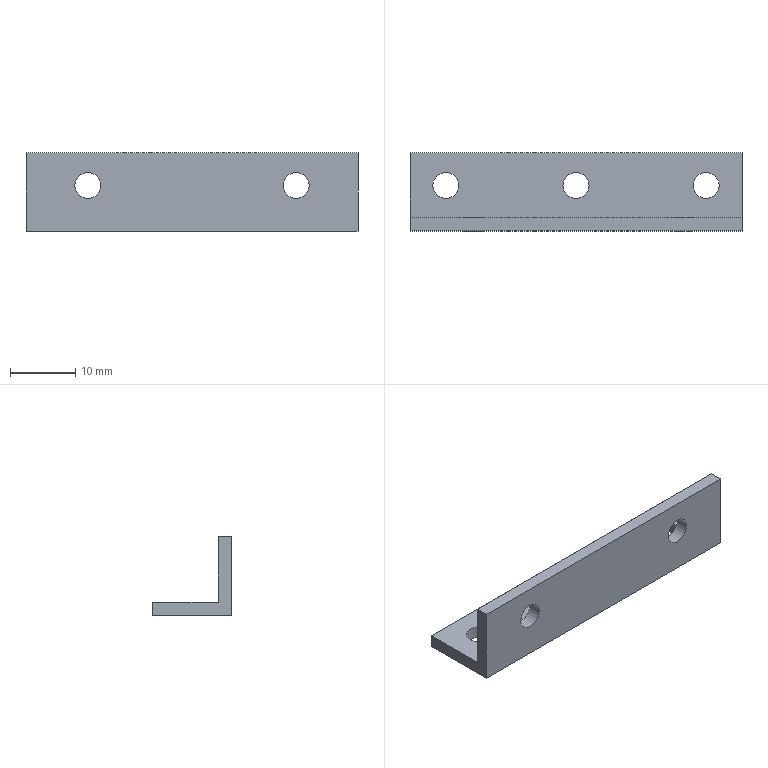Part | STEP file | 1-01.8 | 1 solid | 13 faces | box 51 x 12 x 12 mm | volume 2118 mm3 | plane 8 | cylinder 5 | commonest cylinder face diameters 4 x5
STEP:
#1=CARTESIAN_POINT('',(0.,0.,0.));
#2=DIRECTION('',(0.,0.,1.));
#3=DIRECTION('',(1.,0.,0.));
#4=AXIS2_PLACEMENT_3D('',#1,#2,#3);
#5=CARTESIAN_POINT('',(25.5,-6.,-6.));
#6=VERTEX_POINT('',#5);
#7=CARTESIAN_POINT('',(25.5,6.,-6.));
#8=VERTEX_POINT('',#7);
#9=CARTESIAN_POINT('',(25.5,-6.,-6.));
#10=DIRECTION('',(0.,1.,0.));
#11=VECTOR('',#10,1.);
#12=LINE('',#9,#11);
#13=CARTESIAN_POINT('',(25.5,0.,0.));
#14=DIRECTION('',(1.,0.,0.));
#15=DIRECTION('',(0.,1.,0.));
#16=AXIS2_PLACEMENT_3D('',#13,#14,#15);
#17=PLANE('',#16);
#18=CARTESIAN_POINT('',(-6.,-6.));
#19=DIRECTION('',(1.,0.));
#20=VECTOR('',#19,1.);
#21=LINE('',#18,#20);
#22=(GEOMETRIC_REPRESENTATION_CONTEXT(2)PARAMETRIC_REPRESENTATION_CONTEXT()REPRESENTATION_CONTEXT('',''));
#23=DEFINITIONAL_REPRESENTATION('',(#21),#22);
#24=PCURVE('',#17,#23);
#25=CARTESIAN_POINT('',(0.,0.,-6.));
#26=DIRECTION('',(0.,0.,1.));
#27=DIRECTION('',(0.,1.,0.));
#28=AXIS2_PLACEMENT_3D('',#25,#26,#27);
#29=PLANE('',#28);
#30=CARTESIAN_POINT('',(-6.,-25.5));
#31=DIRECTION('',(1.,0.));
#32=VECTOR('',#31,1.);
#33=LINE('',#30,#32);
#34=(GEOMETRIC_REPRESENTATION_CONTEXT(2)PARAMETRIC_REPRESENTATION_CONTEXT()REPRESENTATION_CONTEXT('',''));
#35=DEFINITIONAL_REPRESENTATION('',(#33),#34);
#36=PCURVE('',#29,#35);
#37=SURFACE_CURVE('',#12,(#24,#36),.PCURVE_S1.);
#38=EDGE_CURVE('',#6,#8,#37,.T.);
#39=ORIENTED_EDGE('',*,*,#38,.T.);
#40=CARTESIAN_POINT('',(25.5,6.,-4.));
#41=VERTEX_POINT('',#40);
#42=CARTESIAN_POINT('',(25.5,6.,-6.));
#43=DIRECTION('',(0.,0.,1.));
#44=VECTOR('',#43,1.);
#45=LINE('',#42,#44);
#46=CARTESIAN_POINT('',(6.,-6.));
#47=DIRECTION('',(0.,1.));
#48=VECTOR('',#47,1.);
#49=LINE('',#46,#48);
#50=(GEOMETRIC_REPRESENTATION_CONTEXT(2)PARAMETRIC_REPRESENTATION_CONTEXT()REPRESENTATION_CONTEXT('',''));
#51=DEFINITIONAL_REPRESENTATION('',(#49),#50);
#52=PCURVE('',#17,#51);
#53=CARTESIAN_POINT('',(0.,6.,-5.));
#54=DIRECTION('',(0.,-1.,0.));
#55=DIRECTION('',(0.,0.,1.));
#56=AXIS2_PLACEMENT_3D('',#53,#54,#55);
#57=PLANE('',#56);
#58=CARTESIAN_POINT('',(-1.,-25.5));
#59=DIRECTION('',(1.,0.));
#60=VECTOR('',#59,1.);
#61=LINE('',#58,#60);
#62=(GEOMETRIC_REPRESENTATION_CONTEXT(2)PARAMETRIC_REPRESENTATION_CONTEXT()REPRESENTATION_CONTEXT('',''));
#63=DEFINITIONAL_REPRESENTATION('',(#61),#62);
#64=PCURVE('',#57,#63);
#65=SURFACE_CURVE('',#45,(#52,#64),.PCURVE_S1.);
#66=EDGE_CURVE('',#8,#41,#65,.T.);
#67=ORIENTED_EDGE('',*,*,#66,.T.);
#68=CARTESIAN_POINT('',(25.5,-4.,-4.));
#69=VERTEX_POINT('',#68);
#70=CARTESIAN_POINT('',(25.5,6.,-4.));
#71=DIRECTION('',(0.,-1.,0.));
#72=VECTOR('',#71,1.);
#73=LINE('',#70,#72);
#74=CARTESIAN_POINT('',(6.,-4.));
#75=DIRECTION('',(-1.,0.));
#76=VECTOR('',#75,1.);
#77=LINE('',#74,#76);
#78=(GEOMETRIC_REPRESENTATION_CONTEXT(2)PARAMETRIC_REPRESENTATION_CONTEXT()REPRESENTATION_CONTEXT('',''));
#79=DEFINITIONAL_REPRESENTATION('',(#77),#78);
#80=PCURVE('',#17,#79);
#81=CARTESIAN_POINT('',(0.,1.,-4.));
#82=DIRECTION('',(0.,0.,-1.));
#83=DIRECTION('',(0.,-1.,0.));
#84=AXIS2_PLACEMENT_3D('',#81,#82,#83);
#85=PLANE('',#84);
#86=CARTESIAN_POINT('',(-5.,-25.5));
#87=DIRECTION('',(1.,0.));
#88=VECTOR('',#87,1.);
#89=LINE('',#86,#88);
#90=(GEOMETRIC_REPRESENTATION_CONTEXT(2)PARAMETRIC_REPRESENTATION_CONTEXT()REPRESENTATION_CONTEXT('',''));
#91=DEFINITIONAL_REPRESENTATION('',(#89),#90);
#92=PCURVE('',#85,#91);
#93=SURFACE_CURVE('',#73,(#80,#92),.PCURVE_S1.);
#94=EDGE_CURVE('',#41,#69,#93,.T.);
#95=ORIENTED_EDGE('',*,*,#94,.T.);
#96=CARTESIAN_POINT('',(25.5,-4.,6.));
#97=VERTEX_POINT('',#96);
#98=CARTESIAN_POINT('',(25.5,-4.,-4.));
#99=DIRECTION('',(0.,0.,1.));
#100=VECTOR('',#99,1.);
#101=LINE('',#98,#100);
#102=CARTESIAN_POINT('',(-4.,-4.));
#103=DIRECTION('',(0.,1.));
#104=VECTOR('',#103,1.);
#105=LINE('',#102,#104);
#106=(GEOMETRIC_REPRESENTATION_CONTEXT(2)PARAMETRIC_REPRESENTATION_CONTEXT()REPRESENTATION_CONTEXT('',''));
#107=DEFINITIONAL_REPRESENTATION('',(#105),#106);
#108=PCURVE('',#17,#107);
#109=CARTESIAN_POINT('',(0.,-4.,1.));
#110=DIRECTION('',(0.,-1.,0.));
#111=DIRECTION('',(0.,0.,1.));
#112=AXIS2_PLACEMENT_3D('',#109,#110,#111);
#113=PLANE('',#112);
#114=CARTESIAN_POINT('',(-5.,-25.5));
#115=DIRECTION('',(1.,0.));
#116=VECTOR('',#115,1.);
#117=LINE('',#114,#116);
#118=(GEOMETRIC_REPRESENTATION_CONTEXT(2)PARAMETRIC_REPRESENTATION_CONTEXT()REPRESENTATION_CONTEXT('',''));
#119=DEFINITIONAL_REPRESENTATION('',(#117),#118);
#120=PCURVE('',#113,#119);
#121=SURFACE_CURVE('',#101,(#108,#120),.PCURVE_S1.);
#122=EDGE_CURVE('',#69,#97,#121,.T.);
#123=ORIENTED_EDGE('',*,*,#122,.T.);
#124=CARTESIAN_POINT('',(25.5,-6.,6.));
#125=VERTEX_POINT('',#124);
#126=CARTESIAN_POINT('',(25.5,-4.,6.));
#127=DIRECTION('',(0.,-1.,0.));
#128=VECTOR('',#127,1.);
#129=LINE('',#126,#128);
#130=CARTESIAN_POINT('',(-4.,6.));
#131=DIRECTION('',(-1.,0.));
#132=VECTOR('',#131,1.);
#133=LINE('',#130,#132);
#134=(GEOMETRIC_REPRESENTATION_CONTEXT(2)PARAMETRIC_REPRESENTATION_CONTEXT()REPRESENTATION_CONTEXT('',''));
#135=DEFINITIONAL_REPRESENTATION('',(#133),#134);
#136=PCURVE('',#17,#135);
#137=CARTESIAN_POINT('',(0.,-5.,6.));
#138=DIRECTION('',(0.,0.,-1.));
#139=DIRECTION('',(0.,-1.,0.));
#140=AXIS2_PLACEMENT_3D('',#137,#138,#139);
#141=PLANE('',#140);
#142=CARTESIAN_POINT('',(-1.,-25.5));
#143=DIRECTION('',(1.,0.));
#144=VECTOR('',#143,1.);
#145=LINE('',#142,#144);
#146=(GEOMETRIC_REPRESENTATION_CONTEXT(2)PARAMETRIC_REPRESENTATION_CONTEXT()REPRESENTATION_CONTEXT('',''));
#147=DEFINITIONAL_REPRESENTATION('',(#145),#146);
#148=PCURVE('',#141,#147);
#149=SURFACE_CURVE('',#129,(#136,#148),.PCURVE_S1.);
#150=EDGE_CURVE('',#97,#125,#149,.T.);
#151=ORIENTED_EDGE('',*,*,#150,.T.);
#152=CARTESIAN_POINT('',(25.5,-6.,6.));
#153=DIRECTION('',(0.,0.,-1.));
#154=VECTOR('',#153,1.);
#155=LINE('',#152,#154);
#156=CARTESIAN_POINT('',(-6.,6.));
#157=DIRECTION('',(0.,-1.));
#158=VECTOR('',#157,1.);
#159=LINE('',#156,#158);
#160=(GEOMETRIC_REPRESENTATION_CONTEXT(2)PARAMETRIC_REPRESENTATION_CONTEXT()REPRESENTATION_CONTEXT('',''));
#161=DEFINITIONAL_REPRESENTATION('',(#159),#160);
#162=PCURVE('',#17,#161);
#163=CARTESIAN_POINT('',(0.,-6.,0.));
#164=DIRECTION('',(0.,1.,0.));
#165=DIRECTION('',(0.,0.,-1.));
#166=AXIS2_PLACEMENT_3D('',#163,#164,#165);
#167=PLANE('',#166);
#168=CARTESIAN_POINT('',(-6.,-25.5));
#169=DIRECTION('',(1.,0.));
#170=VECTOR('',#169,1.);
#171=LINE('',#168,#170);
#172=(GEOMETRIC_REPRESENTATION_CONTEXT(2)PARAMETRIC_REPRESENTATION_CONTEXT()REPRESENTATION_CONTEXT('',''));
#173=DEFINITIONAL_REPRESENTATION('',(#171),#172);
#174=PCURVE('',#167,#173);
#175=SURFACE_CURVE('',#155,(#162,#174),.PCURVE_S1.);
#176=EDGE_CURVE('',#125,#6,#175,.T.);
#177=ORIENTED_EDGE('',*,*,#176,.T.);
#178=EDGE_LOOP('',(#39,#67,#95,#123,#151,#177));
#179=FACE_BOUND('',#178,.T.);
#180=ADVANCED_FACE('',(#179),#17,.T.);
#181=CARTESIAN_POINT('',(-25.5,-6.,-6.));
#182=VERTEX_POINT('',#181);
#183=CARTESIAN_POINT('',(-25.5,6.,-6.));
#184=VERTEX_POINT('',#183);
#185=CARTESIAN_POINT('',(-25.5,-6.,-6.));
#186=DIRECTION('',(0.,1.,0.));
#187=VECTOR('',#186,1.);
#188=LINE('',#185,#187);
#189=CARTESIAN_POINT('',(-25.5,0.,0.));
#190=DIRECTION('',(1.,0.,0.));
#191=DIRECTION('',(0.,1.,0.));
#192=AXIS2_PLACEMENT_3D('',#189,#190,#191);
#193=PLANE('',#192);
#194=CARTESIAN_POINT('',(-6.,-6.));
#195=DIRECTION('',(1.,0.));
#196=VECTOR('',#195,1.);
#197=LINE('',#194,#196);
#198=(GEOMETRIC_REPRESENTATION_CONTEXT(2)PARAMETRIC_REPRESENTATION_CONTEXT()REPRESENTATION_CONTEXT('',''));
#199=DEFINITIONAL_REPRESENTATION('',(#197),#198);
#200=PCURVE('',#193,#199);
#201=CARTESIAN_POINT('',(-6.,25.5));
#202=DIRECTION('',(1.,0.));
#203=VECTOR('',#202,1.);
#204=LINE('',#201,#203);
#205=(GEOMETRIC_REPRESENTATION_CONTEXT(2)PARAMETRIC_REPRESENTATION_CONTEXT()REPRESENTATION_CONTEXT('',''));
#206=DEFINITIONAL_REPRESENTATION('',(#204),#205);
#207=PCURVE('',#29,#206);
#208=SURFACE_CURVE('',#188,(#200,#207),.PCURVE_S1.);
#209=EDGE_CURVE('',#182,#184,#208,.T.);
#210=ORIENTED_EDGE('',*,*,#209,.T.);
#211=CARTESIAN_POINT('',(-25.5,6.,-4.));
#212=VERTEX_POINT('',#211);
#213=CARTESIAN_POINT('',(-25.5,6.,-6.));
#214=DIRECTION('',(0.,0.,1.));
#215=VECTOR('',#214,1.);
#216=LINE('',#213,#215);
#217=CARTESIAN_POINT('',(6.,-6.));
#218=DIRECTION('',(0.,1.));
#219=VECTOR('',#218,1.);
#220=LINE('',#217,#219);
#221=(GEOMETRIC_REPRESENTATION_CONTEXT(2)PARAMETRIC_REPRESENTATION_CONTEXT()REPRESENTATION_CONTEXT('',''));
#222=DEFINITIONAL_REPRESENTATION('',(#220),#221);
#223=PCURVE('',#193,#222);
#224=CARTESIAN_POINT('',(-1.,25.5));
#225=DIRECTION('',(1.,0.));
#226=VECTOR('',#225,1.);
#227=LINE('',#224,#226);
#228=(GEOMETRIC_REPRESENTATION_CONTEXT(2)PARAMETRIC_REPRESENTATION_CONTEXT()REPRESENTATION_CONTEXT('',''));
#229=DEFINITIONAL_REPRESENTATION('',(#227),#228);
#230=PCURVE('',#57,#229);
#231=SURFACE_CURVE('',#216,(#223,#230),.PCURVE_S1.);
#232=EDGE_CURVE('',#184,#212,#231,.T.);
#233=ORIENTED_EDGE('',*,*,#232,.T.);
#234=CARTESIAN_POINT('',(-25.5,-4.,-4.));
#235=VERTEX_POINT('',#234);
#236=CARTESIAN_POINT('',(-25.5,6.,-4.));
#237=DIRECTION('',(0.,-1.,0.));
#238=VECTOR('',#237,1.);
#239=LINE('',#236,#238);
#240=CARTESIAN_POINT('',(6.,-4.));
#241=DIRECTION('',(-1.,0.));
#242=VECTOR('',#241,1.);
#243=LINE('',#240,#242);
#244=(GEOMETRIC_REPRESENTATION_CONTEXT(2)PARAMETRIC_REPRESENTATION_CONTEXT()REPRESENTATION_CONTEXT('',''));
#245=DEFINITIONAL_REPRESENTATION('',(#243),#244);
#246=PCURVE('',#193,#245);
#247=CARTESIAN_POINT('',(-5.,25.5));
#248=DIRECTION('',(1.,0.));
#249=VECTOR('',#248,1.);
#250=LINE('',#247,#249);
#251=(GEOMETRIC_REPRESENTATION_CONTEXT(2)PARAMETRIC_REPRESENTATION_CONTEXT()REPRESENTATION_CONTEXT('',''));
#252=DEFINITIONAL_REPRESENTATION('',(#250),#251);
#253=PCURVE('',#85,#252);
#254=SURFACE_CURVE('',#239,(#246,#253),.PCURVE_S1.);
#255=EDGE_CURVE('',#212,#235,#254,.T.);
#256=ORIENTED_EDGE('',*,*,#255,.T.);
#257=CARTESIAN_POINT('',(-25.5,-4.,6.));
#258=VERTEX_POINT('',#257);
#259=CARTESIAN_POINT('',(-25.5,-4.,-4.));
#260=DIRECTION('',(0.,0.,1.));
#261=VECTOR('',#260,1.);
#262=LINE('',#259,#261);
#263=CARTESIAN_POINT('',(-4.,-4.));
#264=DIRECTION('',(0.,1.));
#265=VECTOR('',#264,1.);
#266=LINE('',#263,#265);
#267=(GEOMETRIC_REPRESENTATION_CONTEXT(2)PARAMETRIC_REPRESENTATION_CONTEXT()REPRESENTATION_CONTEXT('',''));
#268=DEFINITIONAL_REPRESENTATION('',(#266),#267);
#269=PCURVE('',#193,#268);
#270=CARTESIAN_POINT('',(-5.,25.5));
#271=DIRECTION('',(1.,0.));
#272=VECTOR('',#271,1.);
#273=LINE('',#270,#272);
#274=(GEOMETRIC_REPRESENTATION_CONTEXT(2)PARAMETRIC_REPRESENTATION_CONTEXT()REPRESENTATION_CONTEXT('',''));
#275=DEFINITIONAL_REPRESENTATION('',(#273),#274);
#276=PCURVE('',#113,#275);
#277=SURFACE_CURVE('',#262,(#269,#276),.PCURVE_S1.);
#278=EDGE_CURVE('',#235,#258,#277,.T.);
#279=ORIENTED_EDGE('',*,*,#278,.T.);
#280=CARTESIAN_POINT('',(-25.5,-6.,6.));
#281=VERTEX_POINT('',#280);
#282=CARTESIAN_POINT('',(-25.5,-4.,6.));
#283=DIRECTION('',(0.,-1.,0.));
#284=VECTOR('',#283,1.);
#285=LINE('',#282,#284);
#286=CARTESIAN_POINT('',(-4.,6.));
#287=DIRECTION('',(-1.,0.));
#288=VECTOR('',#287,1.);
#289=LINE('',#286,#288);
#290=(GEOMETRIC_REPRESENTATION_CONTEXT(2)PARAMETRIC_REPRESENTATION_CONTEXT()REPRESENTATION_CONTEXT('',''));
#291=DEFINITIONAL_REPRESENTATION('',(#289),#290);
#292=PCURVE('',#193,#291);
#293=CARTESIAN_POINT('',(-1.,25.5));
#294=DIRECTION('',(1.,0.));
#295=VECTOR('',#294,1.);
#296=LINE('',#293,#295);
#297=(GEOMETRIC_REPRESENTATION_CONTEXT(2)PARAMETRIC_REPRESENTATION_CONTEXT()REPRESENTATION_CONTEXT('',''));
#298=DEFINITIONAL_REPRESENTATION('',(#296),#297);
#299=PCURVE('',#141,#298);
#300=SURFACE_CURVE('',#285,(#292,#299),.PCURVE_S1.);
#301=EDGE_CURVE('',#258,#281,#300,.T.);
#302=ORIENTED_EDGE('',*,*,#301,.T.);
#303=CARTESIAN_POINT('',(-25.5,-6.,6.));
#304=DIRECTION('',(0.,0.,-1.));
#305=VECTOR('',#304,1.);
#306=LINE('',#303,#305);
#307=CARTESIAN_POINT('',(-6.,6.));
#308=DIRECTION('',(0.,-1.));
#309=VECTOR('',#308,1.);
#310=LINE('',#307,#309);
#311=(GEOMETRIC_REPRESENTATION_CONTEXT(2)PARAMETRIC_REPRESENTATION_CONTEXT()REPRESENTATION_CONTEXT('',''));
#312=DEFINITIONAL_REPRESENTATION('',(#310),#311);
#313=PCURVE('',#193,#312);
#314=CARTESIAN_POINT('',(-6.,25.5));
#315=DIRECTION('',(1.,0.));
#316=VECTOR('',#315,1.);
#317=LINE('',#314,#316);
#318=(GEOMETRIC_REPRESENTATION_CONTEXT(2)PARAMETRIC_REPRESENTATION_CONTEXT()REPRESENTATION_CONTEXT('',''));
#319=DEFINITIONAL_REPRESENTATION('',(#317),#318);
#320=PCURVE('',#167,#319);
#321=SURFACE_CURVE('',#306,(#313,#320),.PCURVE_S1.);
#322=EDGE_CURVE('',#281,#182,#321,.T.);
#323=ORIENTED_EDGE('',*,*,#322,.T.);
#324=EDGE_LOOP('',(#210,#233,#256,#279,#302,#323));
#325=FACE_BOUND('',#324,.F.);
#326=ADVANCED_FACE('',(#325),#193,.F.);
#327=ORIENTED_EDGE('',*,*,#66,.T.);
#328=CARTESIAN_POINT('',(25.5,6.,-4.));
#329=DIRECTION('',(-1.,0.,0.));
#330=VECTOR('',#329,1.);
#331=LINE('',#328,#330);
#332=CARTESIAN_POINT('',(1.,-25.5));
#333=DIRECTION('',(0.,1.));
#334=VECTOR('',#333,1.);
#335=LINE('',#332,#334);
#336=(GEOMETRIC_REPRESENTATION_CONTEXT(2)PARAMETRIC_REPRESENTATION_CONTEXT()REPRESENTATION_CONTEXT('',''));
#337=DEFINITIONAL_REPRESENTATION('',(#335),#336);
#338=PCURVE('',#57,#337);
#339=CARTESIAN_POINT('',(-5.,-25.5));
#340=DIRECTION('',(0.,1.));
#341=VECTOR('',#340,1.);
#342=LINE('',#339,#341);
#343=(GEOMETRIC_REPRESENTATION_CONTEXT(2)PARAMETRIC_REPRESENTATION_CONTEXT()REPRESENTATION_CONTEXT('',''));
#344=DEFINITIONAL_REPRESENTATION('',(#342),#343);
#345=PCURVE('',#85,#344);
#346=SURFACE_CURVE('',#331,(#338,#345),.PCURVE_S1.);
#347=EDGE_CURVE('',#41,#212,#346,.T.);
#348=ORIENTED_EDGE('',*,*,#347,.T.);
#349=ORIENTED_EDGE('',*,*,#232,.F.);
#350=CARTESIAN_POINT('',(25.5,6.,-6.));
#351=DIRECTION('',(-1.,0.,0.));
#352=VECTOR('',#351,1.);
#353=LINE('',#350,#352);
#354=CARTESIAN_POINT('',(-1.,-25.5));
#355=DIRECTION('',(0.,1.));
#356=VECTOR('',#355,1.);
#357=LINE('',#354,#356);
#358=(GEOMETRIC_REPRESENTATION_CONTEXT(2)PARAMETRIC_REPRESENTATION_CONTEXT()REPRESENTATION_CONTEXT('',''));
#359=DEFINITIONAL_REPRESENTATION('',(#357),#358);
#360=PCURVE('',#57,#359);
#361=CARTESIAN_POINT('',(6.,-25.5));
#362=DIRECTION('',(0.,1.));
#363=VECTOR('',#362,1.);
#364=LINE('',#361,#363);
#365=(GEOMETRIC_REPRESENTATION_CONTEXT(2)PARAMETRIC_REPRESENTATION_CONTEXT()REPRESENTATION_CONTEXT('',''));
#366=DEFINITIONAL_REPRESENTATION('',(#364),#365);
#367=PCURVE('',#29,#366);
#368=SURFACE_CURVE('',#353,(#360,#367),.PCURVE_S1.);
#369=EDGE_CURVE('',#8,#184,#368,.T.);
#370=ORIENTED_EDGE('',*,*,#369,.F.);
#371=EDGE_LOOP('',(#327,#348,#349,#370));
#372=FACE_BOUND('',#371,.F.);
#373=ADVANCED_FACE('',(#372),#57,.F.);
#374=ORIENTED_EDGE('',*,*,#150,.T.);
#375=CARTESIAN_POINT('',(25.5,-6.,6.));
#376=DIRECTION('',(-1.,0.,0.));
#377=VECTOR('',#376,1.);
#378=LINE('',#375,#377);
#379=CARTESIAN_POINT('',(1.,-25.5));
#380=DIRECTION('',(0.,1.));
#381=VECTOR('',#380,1.);
#382=LINE('',#379,#381);
#383=(GEOMETRIC_REPRESENTATION_CONTEXT(2)PARAMETRIC_REPRESENTATION_CONTEXT()REPRESENTATION_CONTEXT('',''));
#384=DEFINITIONAL_REPRESENTATION('',(#382),#383);
#385=PCURVE('',#141,#384);
#386=CARTESIAN_POINT('',(-6.,-25.5));
#387=DIRECTION('',(0.,1.));
#388=VECTOR('',#387,1.);
#389=LINE('',#386,#388);
#390=(GEOMETRIC_REPRESENTATION_CONTEXT(2)PARAMETRIC_REPRESENTATION_CONTEXT()REPRESENTATION_CONTEXT('',''));
#391=DEFINITIONAL_REPRESENTATION('',(#389),#390);
#392=PCURVE('',#167,#391);
#393=SURFACE_CURVE('',#378,(#385,#392),.PCURVE_S1.);
#394=EDGE_CURVE('',#125,#281,#393,.T.);
#395=ORIENTED_EDGE('',*,*,#394,.T.);
#396=ORIENTED_EDGE('',*,*,#301,.F.);
#397=CARTESIAN_POINT('',(25.5,-4.,6.));
#398=DIRECTION('',(-1.,0.,0.));
#399=VECTOR('',#398,1.);
#400=LINE('',#397,#399);
#401=CARTESIAN_POINT('',(-1.,-25.5));
#402=DIRECTION('',(0.,1.));
#403=VECTOR('',#402,1.);
#404=LINE('',#401,#403);
#405=(GEOMETRIC_REPRESENTATION_CONTEXT(2)PARAMETRIC_REPRESENTATION_CONTEXT()REPRESENTATION_CONTEXT('',''));
#406=DEFINITIONAL_REPRESENTATION('',(#404),#405);
#407=PCURVE('',#141,#406);
#408=CARTESIAN_POINT('',(5.,-25.5));
#409=DIRECTION('',(0.,1.));
#410=VECTOR('',#409,1.);
#411=LINE('',#408,#410);
#412=(GEOMETRIC_REPRESENTATION_CONTEXT(2)PARAMETRIC_REPRESENTATION_CONTEXT()REPRESENTATION_CONTEXT('',''));
#413=DEFINITIONAL_REPRESENTATION('',(#411),#412);
#414=PCURVE('',#113,#413);
#415=SURFACE_CURVE('',#400,(#407,#414),.PCURVE_S1.);
#416=EDGE_CURVE('',#97,#258,#415,.T.);
#417=ORIENTED_EDGE('',*,*,#416,.F.);
#418=EDGE_LOOP('',(#374,#395,#396,#417));
#419=FACE_BOUND('',#418,.F.);
#420=ADVANCED_FACE('',(#419),#141,.F.);
#421=ORIENTED_EDGE('',*,*,#122,.T.);
#422=ORIENTED_EDGE('',*,*,#416,.T.);
#423=ORIENTED_EDGE('',*,*,#278,.F.);
#424=CARTESIAN_POINT('',(25.5,-4.,-4.));
#425=DIRECTION('',(-1.,0.,0.));
#426=VECTOR('',#425,1.);
#427=LINE('',#424,#426);
#428=CARTESIAN_POINT('',(-5.,-25.5));
#429=DIRECTION('',(0.,1.));
#430=VECTOR('',#429,1.);
#431=LINE('',#428,#430);
#432=(GEOMETRIC_REPRESENTATION_CONTEXT(2)PARAMETRIC_REPRESENTATION_CONTEXT()REPRESENTATION_CONTEXT('',''));
#433=DEFINITIONAL_REPRESENTATION('',(#431),#432);
#434=PCURVE('',#113,#433);
#435=CARTESIAN_POINT('',(5.,-25.5));
#436=DIRECTION('',(0.,1.));
#437=VECTOR('',#436,1.);
#438=LINE('',#435,#437);
#439=(GEOMETRIC_REPRESENTATION_CONTEXT(2)PARAMETRIC_REPRESENTATION_CONTEXT()REPRESENTATION_CONTEXT('',''));
#440=DEFINITIONAL_REPRESENTATION('',(#438),#439);
#441=PCURVE('',#85,#440);
#442=SURFACE_CURVE('',#427,(#434,#441),.PCURVE_S1.);
#443=EDGE_CURVE('',#69,#235,#442,.T.);
#444=ORIENTED_EDGE('',*,*,#443,.F.);
#445=EDGE_LOOP('',(#421,#422,#423,#444));
#446=FACE_BOUND('',#445,.F.);
#447=CARTESIAN_POINT('',(-14.,-4.,1.));
#448=VERTEX_POINT('',#447);
#449=CARTESIAN_POINT('',(-16.,-4.,1.));
#450=DIRECTION('',(0.,1.,0.));
#451=DIRECTION('',(1.,0.,0.));
#452=AXIS2_PLACEMENT_3D('',#449,#450,#451);
#453=CIRCLE('',#452,2.);
#454=CARTESIAN_POINT('',(0.,14.));
#455=CARTESIAN_POINT('',(-3.464,14.));
#456=CARTESIAN_POINT('',(-1.732,17.));
#457=CARTESIAN_POINT('',(0.,20.));
#458=CARTESIAN_POINT('',(1.732,17.));
#459=CARTESIAN_POINT('',(3.464,14.));
#460=CARTESIAN_POINT('',(0.,14.));
#461=(BOUNDED_CURVE()B_SPLINE_CURVE(2,(#454,#455,#456,#457,#458,#459,#460),.UNSPECIFIED.,.T.,.F.)B_SPLINE_CURVE_WITH_KNOTS((1,2,2,2,2,1),(-2.094,0.,2.094,4.189,6.283,8.378),.UNSPECIFIED.)CURVE()GEOMETRIC_REPRESENTATION_ITEM()RATIONAL_B_SPLINE_CURVE((1.,0.5,1.,0.5,1.,0.5,1.))REPRESENTATION_ITEM(''));
#462=(GEOMETRIC_REPRESENTATION_CONTEXT(2)PARAMETRIC_REPRESENTATION_CONTEXT()REPRESENTATION_CONTEXT('',''));
#463=DEFINITIONAL_REPRESENTATION('',(#461),#462);
#464=PCURVE('',#113,#463);
#465=CARTESIAN_POINT('',(-16.,-25.5,1.));
#466=DIRECTION('',(0.,1.,0.));
#467=DIRECTION('',(1.,0.,0.));
#468=AXIS2_PLACEMENT_3D('',#465,#466,#467);
#469=CYLINDRICAL_SURFACE('',#468,2.);
#470=CARTESIAN_POINT('',(0.,21.5));
#471=DIRECTION('',(1.,0.));
#472=VECTOR('',#471,1.);
#473=LINE('',#470,#472);
#474=(GEOMETRIC_REPRESENTATION_CONTEXT(2)PARAMETRIC_REPRESENTATION_CONTEXT()REPRESENTATION_CONTEXT('',''));
#475=DEFINITIONAL_REPRESENTATION('',(#473),#474);
#476=PCURVE('',#469,#475);
#477=SURFACE_CURVE('',#453,(#464,#476),.PCURVE_S1.);
#478=EDGE_CURVE('',#448,#448,#477,.T.);
#479=ORIENTED_EDGE('',*,*,#478,.T.);
#480=EDGE_LOOP('',(#479));
#481=FACE_BOUND('',#480,.F.);
#482=CARTESIAN_POINT('',(18.,-4.,1.));
#483=VERTEX_POINT('',#482);
#484=CARTESIAN_POINT('',(16.,-4.,1.));
#485=DIRECTION('',(0.,1.,0.));
#486=DIRECTION('',(1.,0.,0.));
#487=AXIS2_PLACEMENT_3D('',#484,#485,#486);
#488=CIRCLE('',#487,2.);
#489=CARTESIAN_POINT('',(0.,-18.));
#490=CARTESIAN_POINT('',(-3.464,-18.));
#491=CARTESIAN_POINT('',(-1.732,-15.));
#492=CARTESIAN_POINT('',(0.,-12.));
#493=CARTESIAN_POINT('',(1.732,-15.));
#494=CARTESIAN_POINT('',(3.464,-18.));
#495=CARTESIAN_POINT('',(0.,-18.));
#496=(BOUNDED_CURVE()B_SPLINE_CURVE(2,(#489,#490,#491,#492,#493,#494,#495),.UNSPECIFIED.,.T.,.F.)B_SPLINE_CURVE_WITH_KNOTS((1,2,2,2,2,1),(-2.094,0.,2.094,4.189,6.283,8.378),.UNSPECIFIED.)CURVE()GEOMETRIC_REPRESENTATION_ITEM()RATIONAL_B_SPLINE_CURVE((1.,0.5,1.,0.5,1.,0.5,1.))REPRESENTATION_ITEM(''));
#497=(GEOMETRIC_REPRESENTATION_CONTEXT(2)PARAMETRIC_REPRESENTATION_CONTEXT()REPRESENTATION_CONTEXT('',''));
#498=DEFINITIONAL_REPRESENTATION('',(#496),#497);
#499=PCURVE('',#113,#498);
#500=CARTESIAN_POINT('',(16.,-25.5,1.));
#501=DIRECTION('',(0.,1.,0.));
#502=DIRECTION('',(1.,0.,0.));
#503=AXIS2_PLACEMENT_3D('',#500,#501,#502);
#504=CYLINDRICAL_SURFACE('',#503,2.);
#505=CARTESIAN_POINT('',(0.,21.5));
#506=DIRECTION('',(1.,0.));
#507=VECTOR('',#506,1.);
#508=LINE('',#505,#507);
#509=(GEOMETRIC_REPRESENTATION_CONTEXT(2)PARAMETRIC_REPRESENTATION_CONTEXT()REPRESENTATION_CONTEXT('',''));
#510=DEFINITIONAL_REPRESENTATION('',(#508),#509);
#511=PCURVE('',#504,#510);
#512=SURFACE_CURVE('',#488,(#499,#511),.PCURVE_S1.);
#513=EDGE_CURVE('',#483,#483,#512,.T.);
#514=ORIENTED_EDGE('',*,*,#513,.T.);
#515=EDGE_LOOP('',(#514));
#516=FACE_BOUND('',#515,.F.);
#517=ADVANCED_FACE('',(#446,#481,#516),#113,.F.);
#518=ORIENTED_EDGE('',*,*,#176,.T.);
#519=CARTESIAN_POINT('',(25.5,-6.,-6.));
#520=DIRECTION('',(-1.,0.,0.));
#521=VECTOR('',#520,1.);
#522=LINE('',#519,#521);
#523=CARTESIAN_POINT('',(6.,-25.5));
#524=DIRECTION('',(0.,1.));
#525=VECTOR('',#524,1.);
#526=LINE('',#523,#525);
#527=(GEOMETRIC_REPRESENTATION_CONTEXT(2)PARAMETRIC_REPRESENTATION_CONTEXT()REPRESENTATION_CONTEXT('',''));
#528=DEFINITIONAL_REPRESENTATION('',(#526),#527);
#529=PCURVE('',#167,#528);
#530=CARTESIAN_POINT('',(-6.,-25.5));
#531=DIRECTION('',(0.,1.));
#532=VECTOR('',#531,1.);
#533=LINE('',#530,#532);
#534=(GEOMETRIC_REPRESENTATION_CONTEXT(2)PARAMETRIC_REPRESENTATION_CONTEXT()REPRESENTATION_CONTEXT('',''));
#535=DEFINITIONAL_REPRESENTATION('',(#533),#534);
#536=PCURVE('',#29,#535);
#537=SURFACE_CURVE('',#522,(#529,#536),.PCURVE_S1.);
#538=EDGE_CURVE('',#6,#182,#537,.T.);
#539=ORIENTED_EDGE('',*,*,#538,.T.);
#540=ORIENTED_EDGE('',*,*,#322,.F.);
#541=ORIENTED_EDGE('',*,*,#394,.F.);
#542=EDGE_LOOP('',(#518,#539,#540,#541));
#543=FACE_BOUND('',#542,.F.);
#544=CARTESIAN_POINT('',(-14.,-6.,1.));
#545=VERTEX_POINT('',#544);
#546=CARTESIAN_POINT('',(-16.,-6.,1.));
#547=DIRECTION('',(0.,-1.,0.));
#548=DIRECTION('',(1.,0.,0.));
#549=AXIS2_PLACEMENT_3D('',#546,#547,#548);
#550=CIRCLE('',#549,2.);
#551=CARTESIAN_POINT('',(-1.,14.));
#552=CARTESIAN_POINT('',(-4.464,14.));
#553=CARTESIAN_POINT('',(-2.732,17.));
#554=CARTESIAN_POINT('',(-1.,20.));
#555=CARTESIAN_POINT('',(0.7321,17.));
#556=CARTESIAN_POINT('',(2.464,14.));
#557=CARTESIAN_POINT('',(-1.,14.));
#558=(BOUNDED_CURVE()B_SPLINE_CURVE(2,(#551,#552,#553,#554,#555,#556,#557),.UNSPECIFIED.,.T.,.F.)B_SPLINE_CURVE_WITH_KNOTS((1,2,2,2,2,1),(-2.094,0.,2.094,4.189,6.283,8.378),.UNSPECIFIED.)CURVE()GEOMETRIC_REPRESENTATION_ITEM()RATIONAL_B_SPLINE_CURVE((1.,0.5,1.,0.5,1.,0.5,1.))REPRESENTATION_ITEM(''));
#559=(GEOMETRIC_REPRESENTATION_CONTEXT(2)PARAMETRIC_REPRESENTATION_CONTEXT()REPRESENTATION_CONTEXT('',''));
#560=DEFINITIONAL_REPRESENTATION('',(#558),#559);
#561=PCURVE('',#167,#560);
#562=CARTESIAN_POINT('',(6.283,19.5));
#563=DIRECTION('',(-1.,0.));
#564=VECTOR('',#563,1.);
#565=LINE('',#562,#564);
#566=(GEOMETRIC_REPRESENTATION_CONTEXT(2)PARAMETRIC_REPRESENTATION_CONTEXT()REPRESENTATION_CONTEXT('',''));
#567=DEFINITIONAL_REPRESENTATION('',(#565),#566);
#568=PCURVE('',#469,#567);
#569=SURFACE_CURVE('',#550,(#561,#568),.PCURVE_S1.);
#570=EDGE_CURVE('',#545,#545,#569,.T.);
#571=ORIENTED_EDGE('',*,*,#570,.T.);
#572=EDGE_LOOP('',(#571));
#573=FACE_BOUND('',#572,.F.);
#574=CARTESIAN_POINT('',(18.,-6.,1.));
#575=VERTEX_POINT('',#574);
#576=CARTESIAN_POINT('',(16.,-6.,1.));
#577=DIRECTION('',(0.,-1.,0.));
#578=DIRECTION('',(1.,0.,0.));
#579=AXIS2_PLACEMENT_3D('',#576,#577,#578);
#580=CIRCLE('',#579,2.);
#581=CARTESIAN_POINT('',(-1.,-18.));
#582=CARTESIAN_POINT('',(-4.464,-18.));
#583=CARTESIAN_POINT('',(-2.732,-15.));
#584=CARTESIAN_POINT('',(-1.,-12.));
#585=CARTESIAN_POINT('',(0.7321,-15.));
#586=CARTESIAN_POINT('',(2.464,-18.));
#587=CARTESIAN_POINT('',(-1.,-18.));
#588=(BOUNDED_CURVE()B_SPLINE_CURVE(2,(#581,#582,#583,#584,#585,#586,#587),.UNSPECIFIED.,.T.,.F.)B_SPLINE_CURVE_WITH_KNOTS((1,2,2,2,2,1),(-2.094,0.,2.094,4.189,6.283,8.378),.UNSPECIFIED.)CURVE()GEOMETRIC_REPRESENTATION_ITEM()RATIONAL_B_SPLINE_CURVE((1.,0.5,1.,0.5,1.,0.5,1.))REPRESENTATION_ITEM(''));
#589=(GEOMETRIC_REPRESENTATION_CONTEXT(2)PARAMETRIC_REPRESENTATION_CONTEXT()REPRESENTATION_CONTEXT('',''));
#590=DEFINITIONAL_REPRESENTATION('',(#588),#589);
#591=PCURVE('',#167,#590);
#592=CARTESIAN_POINT('',(6.283,19.5));
#593=DIRECTION('',(-1.,0.));
#594=VECTOR('',#593,1.);
#595=LINE('',#592,#594);
#596=(GEOMETRIC_REPRESENTATION_CONTEXT(2)PARAMETRIC_REPRESENTATION_CONTEXT()REPRESENTATION_CONTEXT('',''));
#597=DEFINITIONAL_REPRESENTATION('',(#595),#596);
#598=PCURVE('',#504,#597);
#599=SURFACE_CURVE('',#580,(#591,#598),.PCURVE_S1.);
#600=EDGE_CURVE('',#575,#575,#599,.T.);
#601=ORIENTED_EDGE('',*,*,#600,.T.);
#602=EDGE_LOOP('',(#601));
#603=FACE_BOUND('',#602,.F.);
#604=ADVANCED_FACE('',(#543,#573,#603),#167,.F.);
#605=ORIENTED_EDGE('',*,*,#570,.F.);
#606=CARTESIAN_POINT('',(-14.,-6.,1.));
#607=DIRECTION('',(0.,1.,0.));
#608=VECTOR('',#607,1.);
#609=LINE('',#606,#608);
#610=CARTESIAN_POINT('',(6.283,19.5));
#611=DIRECTION('',(0.,1.));
#612=VECTOR('',#611,1.);
#613=LINE('',#610,#612);
#614=(GEOMETRIC_REPRESENTATION_CONTEXT(2)PARAMETRIC_REPRESENTATION_CONTEXT()REPRESENTATION_CONTEXT('',''));
#615=DEFINITIONAL_REPRESENTATION('',(#613),#614);
#616=PCURVE('',#469,#615);
#617=CARTESIAN_POINT('',(0.,19.5));
#618=DIRECTION('',(0.,1.));
#619=VECTOR('',#618,1.);
#620=LINE('',#617,#619);
#621=(GEOMETRIC_REPRESENTATION_CONTEXT(2)PARAMETRIC_REPRESENTATION_CONTEXT()REPRESENTATION_CONTEXT('',''));
#622=DEFINITIONAL_REPRESENTATION('',(#620),#621);
#623=PCURVE('',#469,#622);
#624=SEAM_CURVE('',#609,(#616,#623),.PCURVE_S1.);
#625=EDGE_CURVE('',#545,#448,#624,.T.);
#626=ORIENTED_EDGE('',*,*,#625,.T.);
#627=ORIENTED_EDGE('',*,*,#478,.F.);
#628=ORIENTED_EDGE('',*,*,#625,.F.);
#629=EDGE_LOOP('',(#605,#626,#627,#628));
#630=FACE_BOUND('',#629,.F.);
#631=ADVANCED_FACE('',(#630),#469,.F.);
#632=ORIENTED_EDGE('',*,*,#600,.F.);
#633=CARTESIAN_POINT('',(18.,-6.,1.));
#634=DIRECTION('',(0.,1.,0.));
#635=VECTOR('',#634,1.);
#636=LINE('',#633,#635);
#637=CARTESIAN_POINT('',(6.283,19.5));
#638=DIRECTION('',(0.,1.));
#639=VECTOR('',#638,1.);
#640=LINE('',#637,#639);
#641=(GEOMETRIC_REPRESENTATION_CONTEXT(2)PARAMETRIC_REPRESENTATION_CONTEXT()REPRESENTATION_CONTEXT('',''));
#642=DEFINITIONAL_REPRESENTATION('',(#640),#641);
#643=PCURVE('',#504,#642);
#644=CARTESIAN_POINT('',(0.,19.5));
#645=DIRECTION('',(0.,1.));
#646=VECTOR('',#645,1.);
#647=LINE('',#644,#646);
#648=(GEOMETRIC_REPRESENTATION_CONTEXT(2)PARAMETRIC_REPRESENTATION_CONTEXT()REPRESENTATION_CONTEXT('',''));
#649=DEFINITIONAL_REPRESENTATION('',(#647),#648);
#650=PCURVE('',#504,#649);
#651=SEAM_CURVE('',#636,(#643,#650),.PCURVE_S1.);
#652=EDGE_CURVE('',#575,#483,#651,.T.);
#653=ORIENTED_EDGE('',*,*,#652,.T.);
#654=ORIENTED_EDGE('',*,*,#513,.F.);
#655=ORIENTED_EDGE('',*,*,#652,.F.);
#656=EDGE_LOOP('',(#632,#653,#654,#655));
#657=FACE_BOUND('',#656,.F.);
#658=ADVANCED_FACE('',(#657),#504,.F.);
#659=ORIENTED_EDGE('',*,*,#38,.T.);
#660=ORIENTED_EDGE('',*,*,#369,.T.);
#661=ORIENTED_EDGE('',*,*,#209,.F.);
#662=ORIENTED_EDGE('',*,*,#538,.F.);
#663=EDGE_LOOP('',(#659,#660,#661,#662));
#664=FACE_BOUND('',#663,.F.);
#665=CARTESIAN_POINT('',(22.,1.,-6.));
#666=VERTEX_POINT('',#665);
#667=CARTESIAN_POINT('',(20.,1.,-6.));
#668=DIRECTION('',(0.,0.,-1.));
#669=DIRECTION('',(1.,0.,0.));
#670=AXIS2_PLACEMENT_3D('',#667,#668,#669);
#671=CIRCLE('',#670,2.);
#672=CARTESIAN_POINT('',(1.,-22.));
#673=CARTESIAN_POINT('',(-2.464,-22.));
#674=CARTESIAN_POINT('',(-0.7321,-19.));
#675=CARTESIAN_POINT('',(1.,-16.));
#676=CARTESIAN_POINT('',(2.732,-19.));
#677=CARTESIAN_POINT('',(4.464,-22.));
#678=CARTESIAN_POINT('',(1.,-22.));
#679=(BOUNDED_CURVE()B_SPLINE_CURVE(2,(#672,#673,#674,#675,#676,#677,#678),.UNSPECIFIED.,.T.,.F.)B_SPLINE_CURVE_WITH_KNOTS((1,2,2,2,2,1),(-2.094,0.,2.094,4.189,6.283,8.378),.UNSPECIFIED.)CURVE()GEOMETRIC_REPRESENTATION_ITEM()RATIONAL_B_SPLINE_CURVE((1.,0.5,1.,0.5,1.,0.5,1.))REPRESENTATION_ITEM(''));
#680=(GEOMETRIC_REPRESENTATION_CONTEXT(2)PARAMETRIC_REPRESENTATION_CONTEXT()REPRESENTATION_CONTEXT('',''));
#681=DEFINITIONAL_REPRESENTATION('',(#679),#680);
#682=PCURVE('',#29,#681);
#683=CARTESIAN_POINT('',(20.,1.,25.5));
#684=DIRECTION('',(0.,0.,-1.));
#685=DIRECTION('',(1.,0.,0.));
#686=AXIS2_PLACEMENT_3D('',#683,#684,#685);
#687=CYLINDRICAL_SURFACE('',#686,2.);
#688=CARTESIAN_POINT('',(0.,31.5));
#689=DIRECTION('',(1.,0.));
#690=VECTOR('',#689,1.);
#691=LINE('',#688,#690);
#692=(GEOMETRIC_REPRESENTATION_CONTEXT(2)PARAMETRIC_REPRESENTATION_CONTEXT()REPRESENTATION_CONTEXT('',''));
#693=DEFINITIONAL_REPRESENTATION('',(#691),#692);
#694=PCURVE('',#687,#693);
#695=SURFACE_CURVE('',#671,(#682,#694),.PCURVE_S1.);
#696=EDGE_CURVE('',#666,#666,#695,.T.);
#697=ORIENTED_EDGE('',*,*,#696,.T.);
#698=EDGE_LOOP('',(#697));
#699=FACE_BOUND('',#698,.F.);
#700=CARTESIAN_POINT('',(-18.,1.,-6.));
#701=VERTEX_POINT('',#700);
#702=CARTESIAN_POINT('',(-20.,1.,-6.));
#703=DIRECTION('',(0.,0.,-1.));
#704=DIRECTION('',(1.,0.,0.));
#705=AXIS2_PLACEMENT_3D('',#702,#703,#704);
#706=CIRCLE('',#705,2.);
#707=CARTESIAN_POINT('',(1.,18.));
#708=CARTESIAN_POINT('',(-2.464,18.));
#709=CARTESIAN_POINT('',(-0.7321,21.));
#710=CARTESIAN_POINT('',(1.,24.));
#711=CARTESIAN_POINT('',(2.732,21.));
#712=CARTESIAN_POINT('',(4.464,18.));
#713=CARTESIAN_POINT('',(1.,18.));
#714=(BOUNDED_CURVE()B_SPLINE_CURVE(2,(#707,#708,#709,#710,#711,#712,#713),.UNSPECIFIED.,.T.,.F.)B_SPLINE_CURVE_WITH_KNOTS((1,2,2,2,2,1),(-2.094,0.,2.094,4.189,6.283,8.378),.UNSPECIFIED.)CURVE()GEOMETRIC_REPRESENTATION_ITEM()RATIONAL_B_SPLINE_CURVE((1.,0.5,1.,0.5,1.,0.5,1.))REPRESENTATION_ITEM(''));
#715=(GEOMETRIC_REPRESENTATION_CONTEXT(2)PARAMETRIC_REPRESENTATION_CONTEXT()REPRESENTATION_CONTEXT('',''));
#716=DEFINITIONAL_REPRESENTATION('',(#714),#715);
#717=PCURVE('',#29,#716);
#718=CARTESIAN_POINT('',(-20.,1.,25.5));
#719=DIRECTION('',(0.,0.,-1.));
#720=DIRECTION('',(1.,0.,0.));
#721=AXIS2_PLACEMENT_3D('',#718,#719,#720);
#722=CYLINDRICAL_SURFACE('',#721,2.);
#723=CARTESIAN_POINT('',(0.,31.5));
#724=DIRECTION('',(1.,0.));
#725=VECTOR('',#724,1.);
#726=LINE('',#723,#725);
#727=(GEOMETRIC_REPRESENTATION_CONTEXT(2)PARAMETRIC_REPRESENTATION_CONTEXT()REPRESENTATION_CONTEXT('',''));
#728=DEFINITIONAL_REPRESENTATION('',(#726),#727);
#729=PCURVE('',#722,#728);
#730=SURFACE_CURVE('',#706,(#717,#729),.PCURVE_S1.);
#731=EDGE_CURVE('',#701,#701,#730,.T.);
#732=ORIENTED_EDGE('',*,*,#731,.T.);
#733=EDGE_LOOP('',(#732));
#734=FACE_BOUND('',#733,.F.);
#735=CARTESIAN_POINT('',(2.,1.,-6.));
#736=VERTEX_POINT('',#735);
#737=CARTESIAN_POINT('',(0.,1.,-6.));
#738=DIRECTION('',(0.,0.,-1.));
#739=DIRECTION('',(1.,0.,0.));
#740=AXIS2_PLACEMENT_3D('',#737,#738,#739);
#741=CIRCLE('',#740,2.);
#742=CARTESIAN_POINT('',(1.,-2.));
#743=CARTESIAN_POINT('',(-2.464,-2.));
#744=CARTESIAN_POINT('',(-0.7321,1.));
#745=CARTESIAN_POINT('',(1.,4.));
#746=CARTESIAN_POINT('',(2.732,1.));
#747=CARTESIAN_POINT('',(4.464,-2.));
#748=CARTESIAN_POINT('',(1.,-2.));
#749=(BOUNDED_CURVE()B_SPLINE_CURVE(2,(#742,#743,#744,#745,#746,#747,#748),.UNSPECIFIED.,.T.,.F.)B_SPLINE_CURVE_WITH_KNOTS((1,2,2,2,2,1),(-2.094,0.,2.094,4.189,6.283,8.378),.UNSPECIFIED.)CURVE()GEOMETRIC_REPRESENTATION_ITEM()RATIONAL_B_SPLINE_CURVE((1.,0.5,1.,0.5,1.,0.5,1.))REPRESENTATION_ITEM(''));
#750=(GEOMETRIC_REPRESENTATION_CONTEXT(2)PARAMETRIC_REPRESENTATION_CONTEXT()REPRESENTATION_CONTEXT('',''));
#751=DEFINITIONAL_REPRESENTATION('',(#749),#750);
#752=PCURVE('',#29,#751);
#753=CARTESIAN_POINT('',(0.,1.,25.5));
#754=DIRECTION('',(0.,0.,-1.));
#755=DIRECTION('',(1.,0.,0.));
#756=AXIS2_PLACEMENT_3D('',#753,#754,#755);
#757=CYLINDRICAL_SURFACE('',#756,2.);
#758=CARTESIAN_POINT('',(0.,31.5));
#759=DIRECTION('',(1.,0.));
#760=VECTOR('',#759,1.);
#761=LINE('',#758,#760);
#762=(GEOMETRIC_REPRESENTATION_CONTEXT(2)PARAMETRIC_REPRESENTATION_CONTEXT()REPRESENTATION_CONTEXT('',''));
#763=DEFINITIONAL_REPRESENTATION('',(#761),#762);
#764=PCURVE('',#757,#763);
#765=SURFACE_CURVE('',#741,(#752,#764),.PCURVE_S1.);
#766=EDGE_CURVE('',#736,#736,#765,.T.);
#767=ORIENTED_EDGE('',*,*,#766,.T.);
#768=EDGE_LOOP('',(#767));
#769=FACE_BOUND('',#768,.F.);
#770=ADVANCED_FACE('',(#664,#699,#734,#769),#29,.F.);
#771=ORIENTED_EDGE('',*,*,#94,.T.);
#772=ORIENTED_EDGE('',*,*,#443,.T.);
#773=ORIENTED_EDGE('',*,*,#255,.F.);
#774=ORIENTED_EDGE('',*,*,#347,.F.);
#775=EDGE_LOOP('',(#771,#772,#773,#774));
#776=FACE_BOUND('',#775,.F.);
#777=CARTESIAN_POINT('',(22.,1.,-4.));
#778=VERTEX_POINT('',#777);
#779=CARTESIAN_POINT('',(20.,1.,-4.));
#780=DIRECTION('',(0.,0.,1.));
#781=DIRECTION('',(1.,0.,0.));
#782=AXIS2_PLACEMENT_3D('',#779,#780,#781);
#783=CIRCLE('',#782,2.);
#784=CARTESIAN_POINT('',(0.,-22.));
#785=CARTESIAN_POINT('',(-3.464,-22.));
#786=CARTESIAN_POINT('',(-1.732,-19.));
#787=CARTESIAN_POINT('',(0.,-16.));
#788=CARTESIAN_POINT('',(1.732,-19.));
#789=CARTESIAN_POINT('',(3.464,-22.));
#790=CARTESIAN_POINT('',(0.,-22.));
#791=(BOUNDED_CURVE()B_SPLINE_CURVE(2,(#784,#785,#786,#787,#788,#789,#790),.UNSPECIFIED.,.T.,.F.)B_SPLINE_CURVE_WITH_KNOTS((1,2,2,2,2,1),(-2.094,0.,2.094,4.189,6.283,8.378),.UNSPECIFIED.)CURVE()GEOMETRIC_REPRESENTATION_ITEM()RATIONAL_B_SPLINE_CURVE((1.,0.5,1.,0.5,1.,0.5,1.))REPRESENTATION_ITEM(''));
#792=(GEOMETRIC_REPRESENTATION_CONTEXT(2)PARAMETRIC_REPRESENTATION_CONTEXT()REPRESENTATION_CONTEXT('',''));
#793=DEFINITIONAL_REPRESENTATION('',(#791),#792);
#794=PCURVE('',#85,#793);
#795=CARTESIAN_POINT('',(6.283,29.5));
#796=DIRECTION('',(-1.,0.));
#797=VECTOR('',#796,1.);
#798=LINE('',#795,#797);
#799=(GEOMETRIC_REPRESENTATION_CONTEXT(2)PARAMETRIC_REPRESENTATION_CONTEXT()REPRESENTATION_CONTEXT('',''));
#800=DEFINITIONAL_REPRESENTATION('',(#798),#799);
#801=PCURVE('',#687,#800);
#802=SURFACE_CURVE('',#783,(#794,#801),.PCURVE_S1.);
#803=EDGE_CURVE('',#778,#778,#802,.T.);
#804=ORIENTED_EDGE('',*,*,#803,.T.);
#805=EDGE_LOOP('',(#804));
#806=FACE_BOUND('',#805,.F.);
#807=CARTESIAN_POINT('',(-18.,1.,-4.));
#808=VERTEX_POINT('',#807);
#809=CARTESIAN_POINT('',(-20.,1.,-4.));
#810=DIRECTION('',(0.,0.,1.));
#811=DIRECTION('',(1.,0.,0.));
#812=AXIS2_PLACEMENT_3D('',#809,#810,#811);
#813=CIRCLE('',#812,2.);
#814=CARTESIAN_POINT('',(0.,18.));
#815=CARTESIAN_POINT('',(-3.464,18.));
#816=CARTESIAN_POINT('',(-1.732,21.));
#817=CARTESIAN_POINT('',(0.,24.));
#818=CARTESIAN_POINT('',(1.732,21.));
#819=CARTESIAN_POINT('',(3.464,18.));
#820=CARTESIAN_POINT('',(0.,18.));
#821=(BOUNDED_CURVE()B_SPLINE_CURVE(2,(#814,#815,#816,#817,#818,#819,#820),.UNSPECIFIED.,.T.,.F.)B_SPLINE_CURVE_WITH_KNOTS((1,2,2,2,2,1),(-2.094,0.,2.094,4.189,6.283,8.378),.UNSPECIFIED.)CURVE()GEOMETRIC_REPRESENTATION_ITEM()RATIONAL_B_SPLINE_CURVE((1.,0.5,1.,0.5,1.,0.5,1.))REPRESENTATION_ITEM(''));
#822=(GEOMETRIC_REPRESENTATION_CONTEXT(2)PARAMETRIC_REPRESENTATION_CONTEXT()REPRESENTATION_CONTEXT('',''));
#823=DEFINITIONAL_REPRESENTATION('',(#821),#822);
#824=PCURVE('',#85,#823);
#825=CARTESIAN_POINT('',(6.283,29.5));
#826=DIRECTION('',(-1.,0.));
#827=VECTOR('',#826,1.);
#828=LINE('',#825,#827);
#829=(GEOMETRIC_REPRESENTATION_CONTEXT(2)PARAMETRIC_REPRESENTATION_CONTEXT()REPRESENTATION_CONTEXT('',''));
#830=DEFINITIONAL_REPRESENTATION('',(#828),#829);
#831=PCURVE('',#722,#830);
#832=SURFACE_CURVE('',#813,(#824,#831),.PCURVE_S1.);
#833=EDGE_CURVE('',#808,#808,#832,.T.);
#834=ORIENTED_EDGE('',*,*,#833,.T.);
#835=EDGE_LOOP('',(#834));
#836=FACE_BOUND('',#835,.F.);
#837=CARTESIAN_POINT('',(2.,1.,-4.));
#838=VERTEX_POINT('',#837);
#839=CARTESIAN_POINT('',(0.,1.,-4.));
#840=DIRECTION('',(0.,0.,1.));
#841=DIRECTION('',(1.,0.,0.));
#842=AXIS2_PLACEMENT_3D('',#839,#840,#841);
#843=CIRCLE('',#842,2.);
#844=CARTESIAN_POINT('',(0.,-2.));
#845=CARTESIAN_POINT('',(-3.464,-2.));
#846=CARTESIAN_POINT('',(-1.732,1.));
#847=CARTESIAN_POINT('',(0.,4.));
#848=CARTESIAN_POINT('',(1.732,1.));
#849=CARTESIAN_POINT('',(3.464,-2.));
#850=CARTESIAN_POINT('',(0.,-2.));
#851=(BOUNDED_CURVE()B_SPLINE_CURVE(2,(#844,#845,#846,#847,#848,#849,#850),.UNSPECIFIED.,.T.,.F.)B_SPLINE_CURVE_WITH_KNOTS((1,2,2,2,2,1),(-2.094,0.,2.094,4.189,6.283,8.378),.UNSPECIFIED.)CURVE()GEOMETRIC_REPRESENTATION_ITEM()RATIONAL_B_SPLINE_CURVE((1.,0.5,1.,0.5,1.,0.5,1.))REPRESENTATION_ITEM(''));
#852=(GEOMETRIC_REPRESENTATION_CONTEXT(2)PARAMETRIC_REPRESENTATION_CONTEXT()REPRESENTATION_CONTEXT('',''));
#853=DEFINITIONAL_REPRESENTATION('',(#851),#852);
#854=PCURVE('',#85,#853);
#855=CARTESIAN_POINT('',(6.283,29.5));
#856=DIRECTION('',(-1.,0.));
#857=VECTOR('',#856,1.);
#858=LINE('',#855,#857);
#859=(GEOMETRIC_REPRESENTATION_CONTEXT(2)PARAMETRIC_REPRESENTATION_CONTEXT()REPRESENTATION_CONTEXT('',''));
#860=DEFINITIONAL_REPRESENTATION('',(#858),#859);
#861=PCURVE('',#757,#860);
#862=SURFACE_CURVE('',#843,(#854,#861),.PCURVE_S1.);
#863=EDGE_CURVE('',#838,#838,#862,.T.);
#864=ORIENTED_EDGE('',*,*,#863,.T.);
#865=EDGE_LOOP('',(#864));
#866=FACE_BOUND('',#865,.F.);
#867=ADVANCED_FACE('',(#776,#806,#836,#866),#85,.F.);
#868=ORIENTED_EDGE('',*,*,#803,.F.);
#869=CARTESIAN_POINT('',(22.,1.,-4.));
#870=DIRECTION('',(0.,0.,-1.));
#871=VECTOR('',#870,1.);
#872=LINE('',#869,#871);
#873=CARTESIAN_POINT('',(6.283,29.5));
#874=DIRECTION('',(0.,1.));
#875=VECTOR('',#874,1.);
#876=LINE('',#873,#875);
#877=(GEOMETRIC_REPRESENTATION_CONTEXT(2)PARAMETRIC_REPRESENTATION_CONTEXT()REPRESENTATION_CONTEXT('',''));
#878=DEFINITIONAL_REPRESENTATION('',(#876),#877);
#879=PCURVE('',#687,#878);
#880=CARTESIAN_POINT('',(0.,29.5));
#881=DIRECTION('',(0.,1.));
#882=VECTOR('',#881,1.);
#883=LINE('',#880,#882);
#884=(GEOMETRIC_REPRESENTATION_CONTEXT(2)PARAMETRIC_REPRESENTATION_CONTEXT()REPRESENTATION_CONTEXT('',''));
#885=DEFINITIONAL_REPRESENTATION('',(#883),#884);
#886=PCURVE('',#687,#885);
#887=SEAM_CURVE('',#872,(#879,#886),.PCURVE_S1.);
#888=EDGE_CURVE('',#778,#666,#887,.T.);
#889=ORIENTED_EDGE('',*,*,#888,.T.);
#890=ORIENTED_EDGE('',*,*,#696,.F.);
#891=ORIENTED_EDGE('',*,*,#888,.F.);
#892=EDGE_LOOP('',(#868,#889,#890,#891));
#893=FACE_BOUND('',#892,.F.);
#894=ADVANCED_FACE('',(#893),#687,.F.);
#895=ORIENTED_EDGE('',*,*,#833,.F.);
#896=CARTESIAN_POINT('',(-18.,1.,-4.));
#897=DIRECTION('',(0.,0.,-1.));
#898=VECTOR('',#897,1.);
#899=LINE('',#896,#898);
#900=CARTESIAN_POINT('',(6.283,29.5));
#901=DIRECTION('',(0.,1.));
#902=VECTOR('',#901,1.);
#903=LINE('',#900,#902);
#904=(GEOMETRIC_REPRESENTATION_CONTEXT(2)PARAMETRIC_REPRESENTATION_CONTEXT()REPRESENTATION_CONTEXT('',''));
#905=DEFINITIONAL_REPRESENTATION('',(#903),#904);
#906=PCURVE('',#722,#905);
#907=CARTESIAN_POINT('',(0.,29.5));
#908=DIRECTION('',(0.,1.));
#909=VECTOR('',#908,1.);
#910=LINE('',#907,#909);
#911=(GEOMETRIC_REPRESENTATION_CONTEXT(2)PARAMETRIC_REPRESENTATION_CONTEXT()REPRESENTATION_CONTEXT('',''));
#912=DEFINITIONAL_REPRESENTATION('',(#910),#911);
#913=PCURVE('',#722,#912);
#914=SEAM_CURVE('',#899,(#906,#913),.PCURVE_S1.);
#915=EDGE_CURVE('',#808,#701,#914,.T.);
#916=ORIENTED_EDGE('',*,*,#915,.T.);
#917=ORIENTED_EDGE('',*,*,#731,.F.);
#918=ORIENTED_EDGE('',*,*,#915,.F.);
#919=EDGE_LOOP('',(#895,#916,#917,#918));
#920=FACE_BOUND('',#919,.F.);
#921=ADVANCED_FACE('',(#920),#722,.F.);
#922=ORIENTED_EDGE('',*,*,#863,.F.);
#923=CARTESIAN_POINT('',(2.,1.,-4.));
#924=DIRECTION('',(0.,0.,-1.));
#925=VECTOR('',#924,1.);
#926=LINE('',#923,#925);
#927=CARTESIAN_POINT('',(6.283,29.5));
#928=DIRECTION('',(0.,1.));
#929=VECTOR('',#928,1.);
#930=LINE('',#927,#929);
#931=(GEOMETRIC_REPRESENTATION_CONTEXT(2)PARAMETRIC_REPRESENTATION_CONTEXT()REPRESENTATION_CONTEXT('',''));
#932=DEFINITIONAL_REPRESENTATION('',(#930),#931);
#933=PCURVE('',#757,#932);
#934=CARTESIAN_POINT('',(0.,29.5));
#935=DIRECTION('',(0.,1.));
#936=VECTOR('',#935,1.);
#937=LINE('',#934,#936);
#938=(GEOMETRIC_REPRESENTATION_CONTEXT(2)PARAMETRIC_REPRESENTATION_CONTEXT()REPRESENTATION_CONTEXT('',''));
#939=DEFINITIONAL_REPRESENTATION('',(#937),#938);
#940=PCURVE('',#757,#939);
#941=SEAM_CURVE('',#926,(#933,#940),.PCURVE_S1.);
#942=EDGE_CURVE('',#838,#736,#941,.T.);
#943=ORIENTED_EDGE('',*,*,#942,.T.);
#944=ORIENTED_EDGE('',*,*,#766,.F.);
#945=ORIENTED_EDGE('',*,*,#942,.F.);
#946=EDGE_LOOP('',(#922,#943,#944,#945));
#947=FACE_BOUND('',#946,.F.);
#948=ADVANCED_FACE('',(#947),#757,.F.);
#949=CLOSED_SHELL('',(#180,#326,#373,#420,#517,#604,#631,#658,#770,#867,#894,#921,#948));
#950=MANIFOLD_SOLID_BREP('',#949);
#951=(LENGTH_UNIT()NAMED_UNIT(*)SI_UNIT(.MILLI.,.METRE.));
#952=UNCERTAINTY_MEASURE_WITH_UNIT(LENGTH_MEASURE(0.0000001),#951,'','');
#953=(NAMED_UNIT(*)PLANE_ANGLE_UNIT()SI_UNIT($,.RADIAN.));
#954=(NAMED_UNIT(*)SI_UNIT($,.STERADIAN.)SOLID_ANGLE_UNIT());
#955=(GEOMETRIC_REPRESENTATION_CONTEXT(3)GLOBAL_UNCERTAINTY_ASSIGNED_CONTEXT((#952))GLOBAL_UNIT_ASSIGNED_CONTEXT((#951,#953,#954))REPRESENTATION_CONTEXT('',''));
#956=ADVANCED_BREP_SHAPE_REPRESENTATION('',(#4,#950),#955);